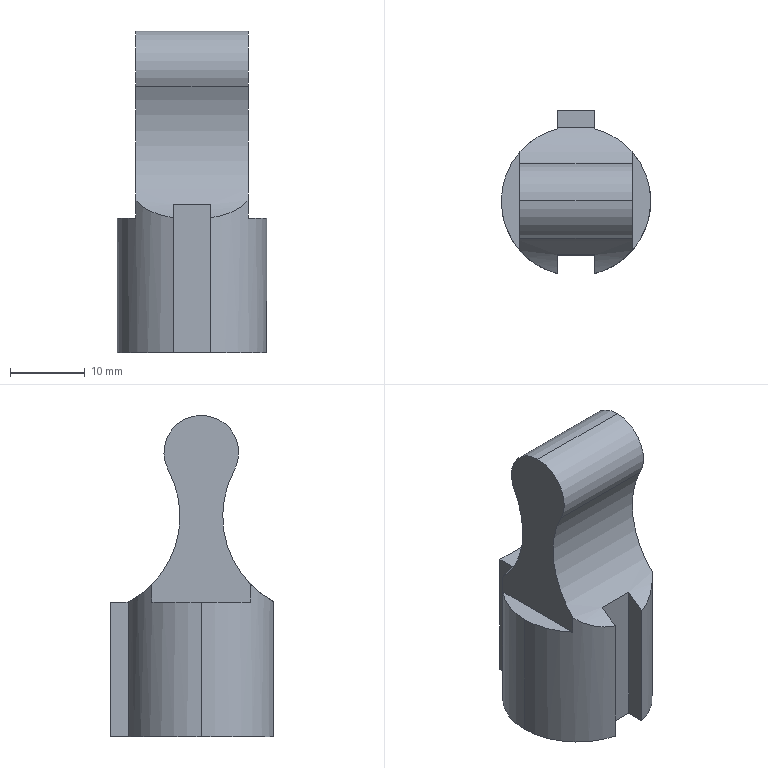Part | STEP file | Seal sleeve 6 | 1 solid | 24 faces | box 20 x 21.865 x 43 mm | volume 7995 mm3 | plane 13 | cylinder 11 | commonest cylinder face diameters 10 x4 20 x3 2.5 x2 26 x2